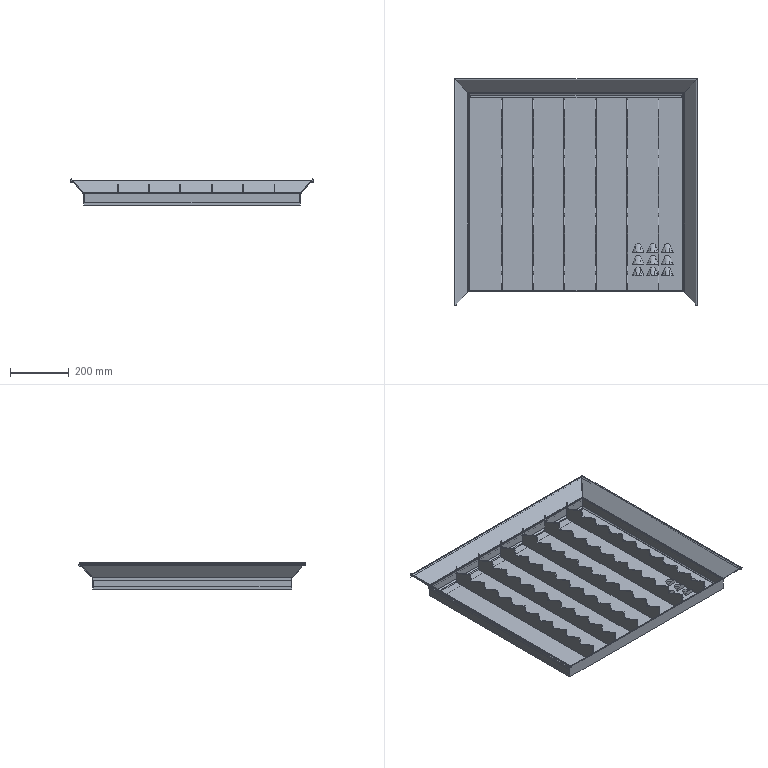Part | SolidWorks | features LayoutProfileFeature 1 | 14 solids | 306 faces | box 829.179 x 774.462 x 88.771 mm | volume 2637561 mm3 | plane 245 | spline 33 | cylinder 28 | commonest cylinder face diameters 2 x8 1 x5 5 x5 10 x4 4 x3 8 x3